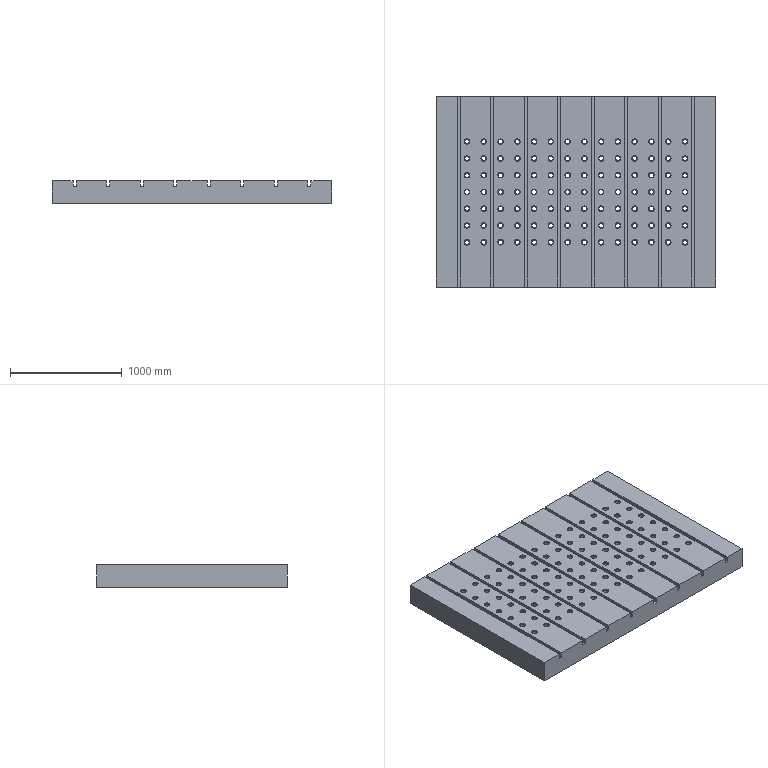Part | NX | features solid 2 | 1 solid | 332 faces | box 2500 x 1700 x 200 mm | volume 806398792 mm3 | cylinder 196 | plane 136 | commonest cylinder face diameters 40 x98 50 x98